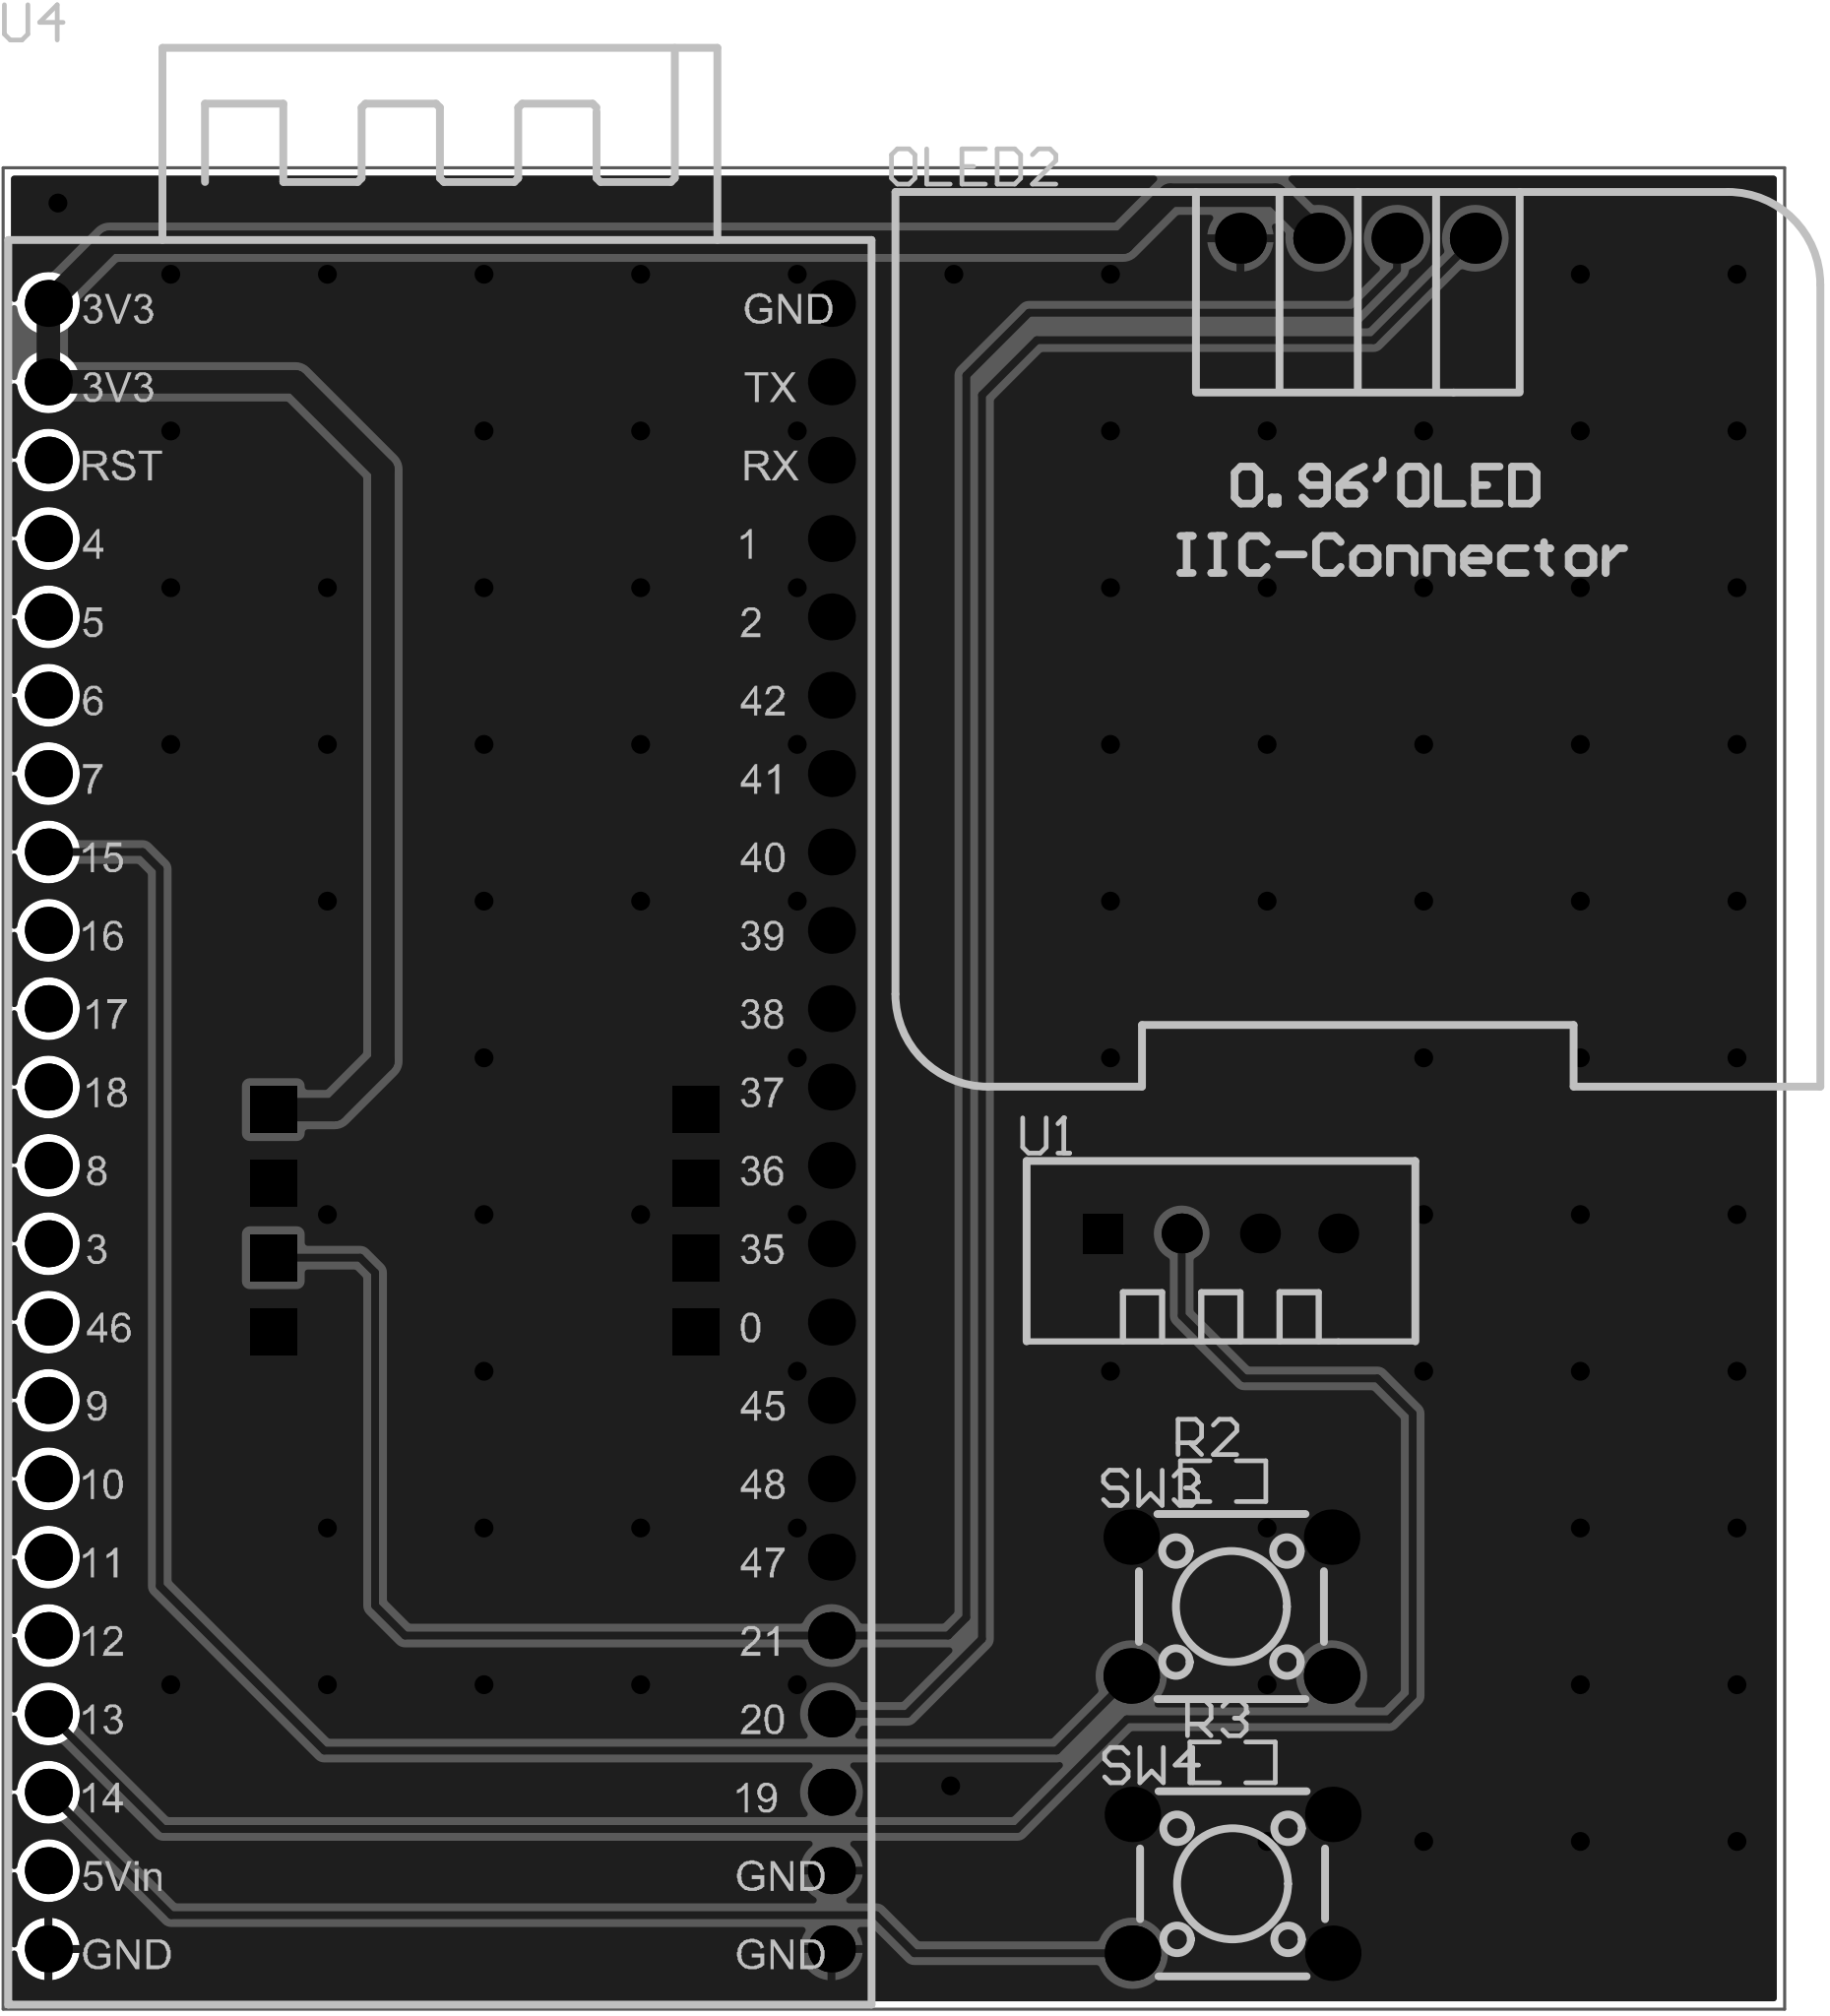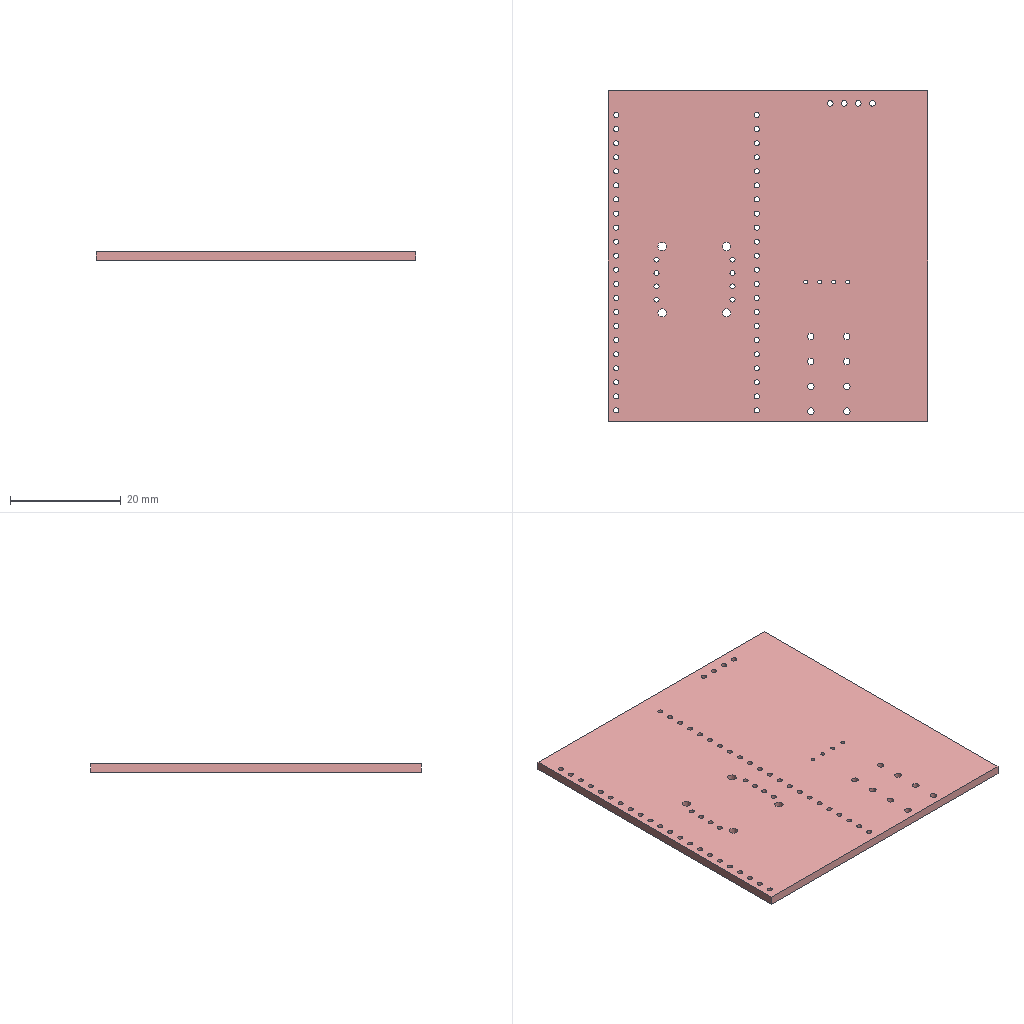Circuit board layout | Altium Designer | box 57.8 x 59.7 x 1.6 mm
Layer stack:
# Altium Designer layer stack of  (unit mm; dielectric type: 0 none, 1 core, 2 prepreg, 3 surface material)
index,name,kind,layer,copper_thickness_mm,dielectric_type,dielectric_thickness_mm,dielectric_material,dielectric_constant
0,Top Paste Mask Layer,other,,,,,,
1,Top Silkscreen Layer,other,,,,,,
2,Top Solder Mask Layer,dielectric,,,3,0.01,,3.3
3,Top Layer,copper,Top Layer,0.035,,,,
4,Dielectric1,dielectric,,,3,1.51,FR4,4.5
5,Bottom Layer,copper,Bottom Layer,0.035,,,,
6,Bottom Solder Mask Layer,dielectric,,,3,0.01,,3.3
7,Bottom Silkscreen Layer,other,,,,,,
8,Bottom Paste Mask Layer,other,,,,,,
# drill layer pairs: low layer,high layer
drill_pair,Top Layer,Bottom Layer
Part placement:
Designator,Comment,Layer,Footprint,Center-X(mm),Center-Y(mm),Rotation
OLED2,,TopLayer,0.96OLED_4P,148.59,155.575,0
R2,10K,TopLayer,R0603,144.22,115.287,0
R3,10K,TopLayer,R0603,144.526,106.172,0
SW3,,TopLayer,SW-TH_4P-L6.0-W6.0-P4.50-LS6.5,144.489,111.223,0
SW4,,TopLayer,SW-TH_4P-L6.0-W6.0-P4.50-LS6.5,144.526,102.235,0
U1,DHT11,TopLayer,SENSOR-TH_DHT11,144.145,123.317,0
U2,MAX30102,BottomLayer,MAX30102,120.269,123.731,270
U4,NO,TopLayer,ESP32S3,118.816,126.793,0
Pad and via stacks:
# Altium Designer via and pad stacks of  (unit mm). Each distinct definition once, with the count of objects using it.
# via: kind,start_layer,end_layer,hole_mm,diameter_mm,mode(0 simple;1 top-mid-bottom;2 full stack),diameter_per_layer,count,example_net
# pad: kind,layer,hole_mm,hole_type(0 round;1 square;2 slot),plating,top_size,top_shape(1 round;2 rect;3 octagon;9 rounded rect),mid_size,bottom_size,mode,footprint,size_per_layer,count,example
pad,Multi-Layer,1,0,plated,1.65x1.65,1,1.65x1.65,1.65x1.65,0,0.96OLED_4P,,4,OLED2.4
pad,Multi-Layer,1.2,0,plated,1.8x1.8,1,1.8x1.8,1.8x1.8,0,SW-TH_4P-L6.0-W6.0-P4.50-LS6.5,,8,SW3.1
pad,Multi-Layer,0.7112,0,plated,1.295x1.295,2,1.295x1.295,1.295x1.295,0,SENSOR-TH_DHT11,,1,U1.1
pad,Multi-Layer,0.7112,0,plated,1.295x1.295,1,1.295x1.295,1.295x1.295,0,SENSOR-TH_DHT11,,3,U1.2
pad,Multi-Layer,0.9144,0,plated,1.524x1.524,2,1.524x1.524,1.524x1.524,0,MAX30102,,8,U2.1
pad,Multi-Layer,0.9144,0,plated,1.524x1.524,1,1.524x1.524,1.524x1.524,0,ESP32S3,,44,U4.1
pad,Top Layer,0,0,plated,0.8065x0.864,2,0.8065x0.864,0.8065x0.864,0,R0603,,4,R2.2
via,Top Layer,Bottom Layer,0.3048,0.61,0,,87,GND
Copper pours:
name,layer,net,type(0 solid;1 hatched;2 none)
Bottom Layer-GND,Bottom Layer,GND,0
Top Layer-GND,Top Layer,GND,0
Design rules, without the lines most boards share:
# Altium Designer design rules of  (exported by Altium Designer, unit mm)
# columns: name | kind | enabled | priority | scope1 | scope2 | descriptor | typed fields (field=value)
Copper_copperRegion_copperThickness1oz | 0 | disabled | 4 | All | All | Clearance Constraint (Gap=5.984mil) (Disabled)(All),(All) | gap=0.152
Copper_copperRegion_copperThickness1oz_1 | 63 | disabled | 4 | All | All | Board Clearance Constraint (Gap=0mil) (Disabled)(All) |
Copper_copperRegion_Copper_copperRegion | 0 | disabled | 5 | All | All | Clearance Constraint (Gap=5.984mil) (Disabled)(All),(All) | gap=0.152
Copper_copperRegion_Copper_copperRegion_1 | 63 | disabled | 5 | All | All | Board Clearance Constraint (Gap=0mil) (Disabled)(All) |
copperThickness1oz | 0 | enabled | 6 | All | All | Clearance Constraint (Gap=5.984mil) (All),(All) | gap=0.152
copperThickness1oz_1 | 63 | enabled | 6 | All | All | Board Clearance Constraint (Gap=0mil) (All) |
copperRegion_copperThickness1oz | 20 | disabled | 1 | All | All | Polygon Connect Rule(Relief Connect )(Conductor Width=10mil) (Relief Angle=90 Angle) (Entries=4) (Air Gap Width=10mil) (Disabled)(All),(All) | connect_style(0=relief,1=direct,2=none)=0 relief_conductor_width=0.254 relief_entries=4
copperRegion_Copper_copperRegion | 20 | disabled | 2 | All | All | Polygon Connect Rule(Relief Connect )(Conductor Width=10mil) (Relief Angle=90 Angle) (Entries=4) (Air Gap Width=10mil) (Disabled)(All),(All) | connect_style(0=relief,1=direct,2=none)=0 relief_conductor_width=0.254 relief_entries=4
copperRegion | 20 | enabled | 3 | All | All | Polygon Connect Rule(Relief Connect )(Conductor Width=10mil) (Relief Angle=90 Angle) (Entries=4) (Air Gap Width=10mil) (All),(All) | connect_style(0=relief,1=direct,2=none)=0 relief_conductor_width=0.254 relief_entries=4